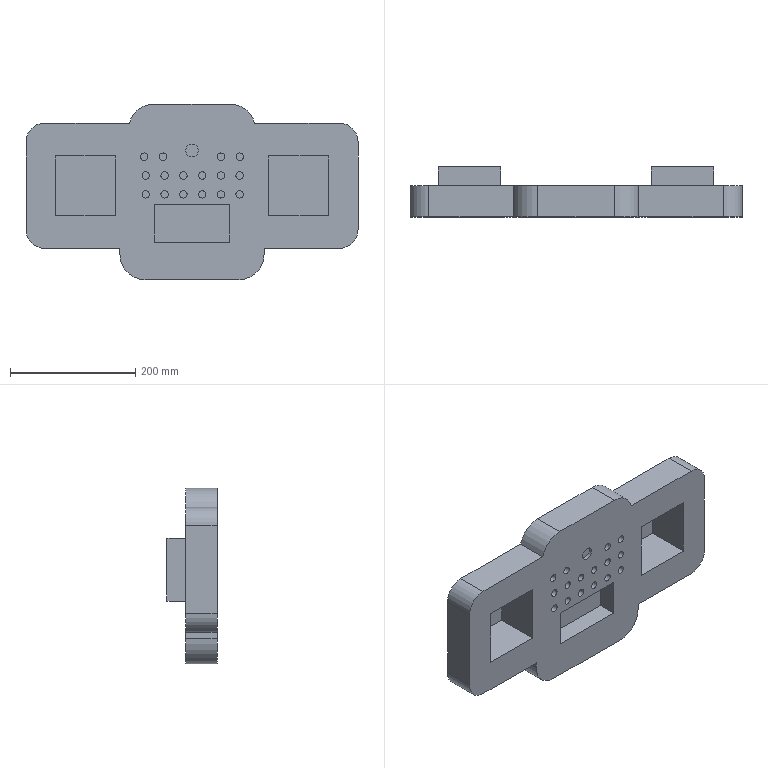Part | STEP file | 111 | 1 solid | 92 faces | box 530 x 80 x 280 mm | volume 5097717 mm3 | plane 61 | cylinder 31 | commonest cylinder face diameters 12 x16 20 x5 60 x4 80 x4 10 x2